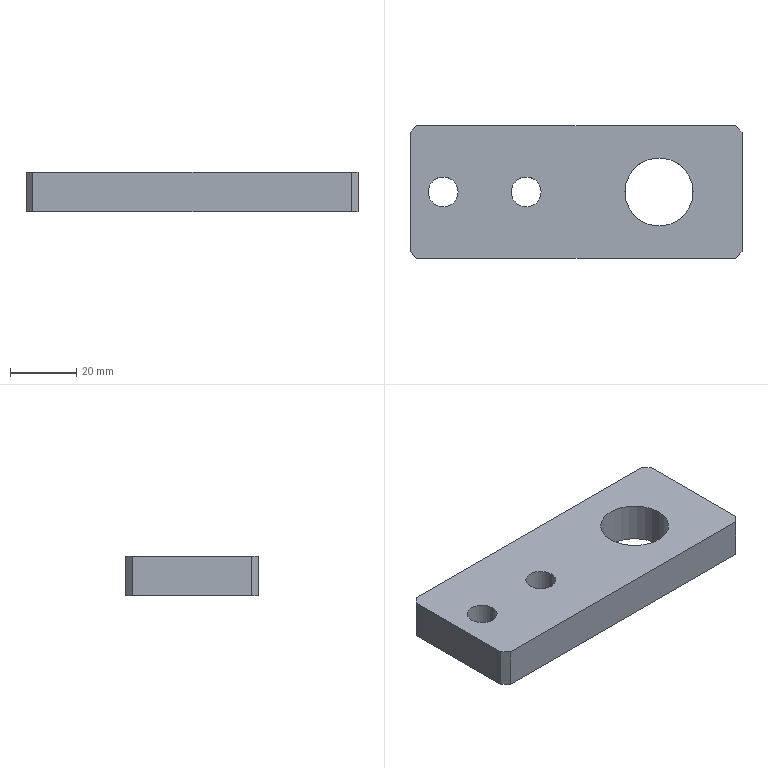Part | SolidWorks | features BaseBody 1 | 1 solid | 16 faces | box 100 x 40 x 12 mm | volume 42416 mm3 | plane 10 | cylinder 6 | commonest cylinder face diameters 9 x4 20.5 x2
STEP:
#1=CARTESIAN_POINT('',(-19.5,0.,0.));
#2=VERTEX_POINT('',#1);
#3=CARTESIAN_POINT('',(-10.5,0.,0.));
#4=VERTEX_POINT('',#3);
#5=CARTESIAN_POINT('',(-15.,0.,0.));
#6=DIRECTION('',(0.,0.,1.));
#7=DIRECTION('',(1.,0.,0.));
#8=AXIS2_PLACEMENT_3D('',#5,#6,#7);
#9=CIRCLE('',#8,4.5);
#10=EDGE_CURVE('',#2,#4,#9,.T.);
#11=ORIENTED_EDGE('',*,*,#10,.F.);
#12=CARTESIAN_POINT('',(-19.5,0.,12.));
#13=VERTEX_POINT('',#12);
#14=CARTESIAN_POINT('',(-19.5,0.,12.));
#15=DIRECTION('',(0.,0.,1.));
#16=VECTOR('',#15,1000.);
#17=LINE('',#14,#16);
#18=EDGE_CURVE('',#2,#13,#17,.T.);
#19=ORIENTED_EDGE('',*,*,#18,.T.);
#20=CARTESIAN_POINT('',(-10.5,0.,12.));
#21=VERTEX_POINT('',#20);
#22=CARTESIAN_POINT('',(-15.,0.,12.));
#23=DIRECTION('',(0.,0.,-1.));
#24=DIRECTION('',(1.,0.,0.));
#25=AXIS2_PLACEMENT_3D('',#22,#23,#24);
#26=CIRCLE('',#25,4.5);
#27=EDGE_CURVE('',#21,#13,#26,.T.);
#28=ORIENTED_EDGE('',*,*,#27,.F.);
#29=CARTESIAN_POINT('',(-10.5,0.,12.));
#30=DIRECTION('',(0.,0.,1.));
#31=VECTOR('',#30,1000.);
#32=LINE('',#29,#31);
#33=EDGE_CURVE('',#4,#21,#32,.T.);
#34=ORIENTED_EDGE('',*,*,#33,.F.);
#35=EDGE_LOOP('',(#11,#19,#28,#34));
#36=FACE_OUTER_BOUND('',#35,.T.);
#37=CARTESIAN_POINT('',(-15.,0.,12.));
#38=DIRECTION('',(0.,0.,1.));
#39=DIRECTION('',(1.,0.,0.));
#40=AXIS2_PLACEMENT_3D('',#37,#38,#39);
#41=CYLINDRICAL_SURFACE('',#40,4.5);
#42=ADVANCED_FACE('',(#36),#41,.F.);
#43=CARTESIAN_POINT('',(-44.5,0.,0.));
#44=VERTEX_POINT('',#43);
#45=CARTESIAN_POINT('',(-35.5,0.,0.));
#46=VERTEX_POINT('',#45);
#47=CARTESIAN_POINT('',(-40.,0.,0.));
#48=DIRECTION('',(0.,0.,1.));
#49=DIRECTION('',(1.,0.,0.));
#50=AXIS2_PLACEMENT_3D('',#47,#48,#49);
#51=CIRCLE('',#50,4.5);
#52=EDGE_CURVE('',#44,#46,#51,.T.);
#53=ORIENTED_EDGE('',*,*,#52,.F.);
#54=CARTESIAN_POINT('',(-44.5,0.,12.));
#55=VERTEX_POINT('',#54);
#56=CARTESIAN_POINT('',(-44.5,0.,12.));
#57=DIRECTION('',(0.,0.,1.));
#58=VECTOR('',#57,1000.);
#59=LINE('',#56,#58);
#60=EDGE_CURVE('',#44,#55,#59,.T.);
#61=ORIENTED_EDGE('',*,*,#60,.T.);
#62=CARTESIAN_POINT('',(-35.5,0.,12.));
#63=VERTEX_POINT('',#62);
#64=CARTESIAN_POINT('',(-40.,0.,12.));
#65=DIRECTION('',(0.,0.,-1.));
#66=DIRECTION('',(1.,0.,0.));
#67=AXIS2_PLACEMENT_3D('',#64,#65,#66);
#68=CIRCLE('',#67,4.5);
#69=EDGE_CURVE('',#63,#55,#68,.T.);
#70=ORIENTED_EDGE('',*,*,#69,.F.);
#71=CARTESIAN_POINT('',(-35.5,0.,12.));
#72=DIRECTION('',(0.,0.,1.));
#73=VECTOR('',#72,1000.);
#74=LINE('',#71,#73);
#75=EDGE_CURVE('',#46,#63,#74,.T.);
#76=ORIENTED_EDGE('',*,*,#75,.F.);
#77=EDGE_LOOP('',(#53,#61,#70,#76));
#78=FACE_OUTER_BOUND('',#77,.T.);
#79=CARTESIAN_POINT('',(-40.,0.,12.));
#80=DIRECTION('',(0.,0.,1.));
#81=DIRECTION('',(1.,0.,0.));
#82=AXIS2_PLACEMENT_3D('',#79,#80,#81);
#83=CYLINDRICAL_SURFACE('',#82,4.5);
#84=ADVANCED_FACE('',(#78),#83,.F.);
#85=CARTESIAN_POINT('',(14.75,0.,0.));
#86=VERTEX_POINT('',#85);
#87=CARTESIAN_POINT('',(35.25,0.,0.));
#88=VERTEX_POINT('',#87);
#89=CARTESIAN_POINT('',(25.,0.,0.));
#90=DIRECTION('',(0.,0.,1.));
#91=DIRECTION('',(1.,0.,0.));
#92=AXIS2_PLACEMENT_3D('',#89,#90,#91);
#93=CIRCLE('',#92,10.25);
#94=EDGE_CURVE('',#86,#88,#93,.T.);
#95=ORIENTED_EDGE('',*,*,#94,.F.);
#96=CARTESIAN_POINT('',(14.75,0.,12.));
#97=VERTEX_POINT('',#96);
#98=CARTESIAN_POINT('',(14.75,0.,12.));
#99=DIRECTION('',(0.,0.,1.));
#100=VECTOR('',#99,1000.);
#101=LINE('',#98,#100);
#102=EDGE_CURVE('',#86,#97,#101,.T.);
#103=ORIENTED_EDGE('',*,*,#102,.T.);
#104=CARTESIAN_POINT('',(35.25,0.,12.));
#105=VERTEX_POINT('',#104);
#106=CARTESIAN_POINT('',(25.,0.,12.));
#107=DIRECTION('',(0.,0.,-1.));
#108=DIRECTION('',(1.,0.,0.));
#109=AXIS2_PLACEMENT_3D('',#106,#107,#108);
#110=CIRCLE('',#109,10.25);
#111=EDGE_CURVE('',#105,#97,#110,.T.);
#112=ORIENTED_EDGE('',*,*,#111,.F.);
#113=CARTESIAN_POINT('',(35.25,0.,12.));
#114=DIRECTION('',(0.,0.,1.));
#115=VECTOR('',#114,1000.);
#116=LINE('',#113,#115);
#117=EDGE_CURVE('',#88,#105,#116,.T.);
#118=ORIENTED_EDGE('',*,*,#117,.F.);
#119=EDGE_LOOP('',(#95,#103,#112,#118));
#120=FACE_OUTER_BOUND('',#119,.T.);
#121=CARTESIAN_POINT('',(25.,0.,12.));
#122=DIRECTION('',(0.,0.,1.));
#123=DIRECTION('',(1.,0.,0.));
#124=AXIS2_PLACEMENT_3D('',#121,#122,#123);
#125=CYLINDRICAL_SURFACE('',#124,10.25);
#126=ADVANCED_FACE('',(#120),#125,.F.);
#127=CARTESIAN_POINT('',(-48.,-20.,12.));
#128=VERTEX_POINT('',#127);
#129=CARTESIAN_POINT('',(48.,-20.,12.));
#130=VERTEX_POINT('',#129);
#131=CARTESIAN_POINT('',(0.,-20.,12.));
#132=DIRECTION('',(1.,0.,0.));
#133=VECTOR('',#132,1000.);
#134=LINE('',#131,#133);
#135=EDGE_CURVE('',#128,#130,#134,.T.);
#136=ORIENTED_EDGE('',*,*,#135,.T.);
#137=CARTESIAN_POINT('',(50.,-18.,12.));
#138=VERTEX_POINT('',#137);
#139=CARTESIAN_POINT('',(48.,-20.,12.));
#140=DIRECTION('',(0.7071,0.7071,0.));
#141=VECTOR('',#140,1000.);
#142=LINE('',#139,#141);
#143=EDGE_CURVE('',#130,#138,#142,.T.);
#144=ORIENTED_EDGE('',*,*,#143,.T.);
#145=CARTESIAN_POINT('',(50.,18.,12.));
#146=VERTEX_POINT('',#145);
#147=CARTESIAN_POINT('',(50.,0.,12.));
#148=DIRECTION('',(0.,1.,0.));
#149=VECTOR('',#148,1000.);
#150=LINE('',#147,#149);
#151=EDGE_CURVE('',#138,#146,#150,.T.);
#152=ORIENTED_EDGE('',*,*,#151,.T.);
#153=CARTESIAN_POINT('',(48.,20.,12.));
#154=VERTEX_POINT('',#153);
#155=CARTESIAN_POINT('',(50.,18.,12.));
#156=DIRECTION('',(-0.7071,0.7071,0.));
#157=VECTOR('',#156,1000.);
#158=LINE('',#155,#157);
#159=EDGE_CURVE('',#146,#154,#158,.T.);
#160=ORIENTED_EDGE('',*,*,#159,.T.);
#161=CARTESIAN_POINT('',(-48.,20.,12.));
#162=VERTEX_POINT('',#161);
#163=CARTESIAN_POINT('',(0.,20.,12.));
#164=DIRECTION('',(-1.,0.,0.));
#165=VECTOR('',#164,1000.);
#166=LINE('',#163,#165);
#167=EDGE_CURVE('',#154,#162,#166,.T.);
#168=ORIENTED_EDGE('',*,*,#167,.T.);
#169=CARTESIAN_POINT('',(-50.,18.,12.));
#170=VERTEX_POINT('',#169);
#171=CARTESIAN_POINT('',(-48.,20.,12.));
#172=DIRECTION('',(-0.7071,-0.7071,0.));
#173=VECTOR('',#172,1000.);
#174=LINE('',#171,#173);
#175=EDGE_CURVE('',#162,#170,#174,.T.);
#176=ORIENTED_EDGE('',*,*,#175,.T.);
#177=CARTESIAN_POINT('',(-50.,-18.,12.));
#178=VERTEX_POINT('',#177);
#179=CARTESIAN_POINT('',(-50.,0.,12.));
#180=DIRECTION('',(0.,-1.,0.));
#181=VECTOR('',#180,1000.);
#182=LINE('',#179,#181);
#183=EDGE_CURVE('',#170,#178,#182,.T.);
#184=ORIENTED_EDGE('',*,*,#183,.T.);
#185=CARTESIAN_POINT('',(-50.,-18.,12.));
#186=DIRECTION('',(0.7071,-0.7071,0.));
#187=VECTOR('',#186,1000.);
#188=LINE('',#185,#187);
#189=EDGE_CURVE('',#178,#128,#188,.T.);
#190=ORIENTED_EDGE('',*,*,#189,.T.);
#191=EDGE_LOOP('',(#136,#144,#152,#160,#168,#176,#184,#190));
#192=FACE_OUTER_BOUND('',#191,.T.);
#193=ORIENTED_EDGE('',*,*,#27,.T.);
#194=CARTESIAN_POINT('',(-15.,0.,12.));
#195=DIRECTION('',(0.,0.,-1.));
#196=DIRECTION('',(1.,0.,0.));
#197=AXIS2_PLACEMENT_3D('',#194,#195,#196);
#198=CIRCLE('',#197,4.5);
#199=EDGE_CURVE('',#13,#21,#198,.T.);
#200=ORIENTED_EDGE('',*,*,#199,.T.);
#201=EDGE_LOOP('',(#193,#200));
#202=FACE_BOUND('',#201,.T.);
#203=ORIENTED_EDGE('',*,*,#69,.T.);
#204=CARTESIAN_POINT('',(-40.,0.,12.));
#205=DIRECTION('',(0.,0.,-1.));
#206=DIRECTION('',(1.,0.,0.));
#207=AXIS2_PLACEMENT_3D('',#204,#205,#206);
#208=CIRCLE('',#207,4.5);
#209=EDGE_CURVE('',#55,#63,#208,.T.);
#210=ORIENTED_EDGE('',*,*,#209,.T.);
#211=EDGE_LOOP('',(#203,#210));
#212=FACE_BOUND('',#211,.T.);
#213=ORIENTED_EDGE('',*,*,#111,.T.);
#214=CARTESIAN_POINT('',(25.,0.,12.));
#215=DIRECTION('',(0.,0.,-1.));
#216=DIRECTION('',(1.,0.,0.));
#217=AXIS2_PLACEMENT_3D('',#214,#215,#216);
#218=CIRCLE('',#217,10.25);
#219=EDGE_CURVE('',#97,#105,#218,.T.);
#220=ORIENTED_EDGE('',*,*,#219,.T.);
#221=EDGE_LOOP('',(#213,#220));
#222=FACE_BOUND('',#221,.T.);
#223=CARTESIAN_POINT('',(0.,0.,12.));
#224=DIRECTION('',(0.,0.,1.));
#225=DIRECTION('',(1.,0.,0.));
#226=AXIS2_PLACEMENT_3D('',#223,#224,#225);
#227=PLANE('',#226);
#228=ADVANCED_FACE('',(#192,#202,#212,#222),#227,.T.);
#229=CARTESIAN_POINT('',(48.,-20.,0.));
#230=VERTEX_POINT('',#229);
#231=CARTESIAN_POINT('',(48.,-20.,12.));
#232=DIRECTION('',(0.,0.,1.));
#233=VECTOR('',#232,1000.);
#234=LINE('',#231,#233);
#235=EDGE_CURVE('',#230,#130,#234,.T.);
#236=ORIENTED_EDGE('',*,*,#235,.F.);
#237=CARTESIAN_POINT('',(50.,-18.,0.));
#238=VERTEX_POINT('',#237);
#239=CARTESIAN_POINT('',(50.,-18.,0.));
#240=DIRECTION('',(-0.7071,-0.7071,0.));
#241=VECTOR('',#240,1000.);
#242=LINE('',#239,#241);
#243=EDGE_CURVE('',#238,#230,#242,.T.);
#244=ORIENTED_EDGE('',*,*,#243,.F.);
#245=CARTESIAN_POINT('',(50.,-18.,12.));
#246=DIRECTION('',(0.,0.,-1.));
#247=VECTOR('',#246,1000.);
#248=LINE('',#245,#247);
#249=EDGE_CURVE('',#138,#238,#248,.T.);
#250=ORIENTED_EDGE('',*,*,#249,.F.);
#251=ORIENTED_EDGE('',*,*,#143,.F.);
#252=EDGE_LOOP('',(#236,#244,#250,#251));
#253=FACE_OUTER_BOUND('',#252,.T.);
#254=CARTESIAN_POINT('',(50.,-18.,12.));
#255=DIRECTION('',(-0.7071,0.7071,0.));
#256=DIRECTION('',(-0.7071,-0.7071,0.));
#257=AXIS2_PLACEMENT_3D('',#254,#255,#256);
#258=PLANE('',#257);
#259=ADVANCED_FACE('',(#253),#258,.F.);
#260=ORIENTED_EDGE('',*,*,#235,.T.);
#261=ORIENTED_EDGE('',*,*,#135,.F.);
#262=CARTESIAN_POINT('',(-48.,-20.,0.));
#263=VERTEX_POINT('',#262);
#264=CARTESIAN_POINT('',(-48.,-20.,12.));
#265=DIRECTION('',(0.,0.,1.));
#266=VECTOR('',#265,1000.);
#267=LINE('',#264,#266);
#268=EDGE_CURVE('',#263,#128,#267,.T.);
#269=ORIENTED_EDGE('',*,*,#268,.F.);
#270=CARTESIAN_POINT('',(-50.,-20.,0.));
#271=DIRECTION('',(-1.,0.,0.));
#272=VECTOR('',#271,1000.);
#273=LINE('',#270,#272);
#274=EDGE_CURVE('',#230,#263,#273,.T.);
#275=ORIENTED_EDGE('',*,*,#274,.F.);
#276=EDGE_LOOP('',(#260,#261,#269,#275));
#277=FACE_OUTER_BOUND('',#276,.T.);
#278=CARTESIAN_POINT('',(-50.,-20.,12.));
#279=DIRECTION('',(0.,1.,0.));
#280=DIRECTION('',(0.,0.,1.));
#281=AXIS2_PLACEMENT_3D('',#278,#279,#280);
#282=PLANE('',#281);
#283=ADVANCED_FACE('',(#277),#282,.F.);
#284=CARTESIAN_POINT('',(-50.,-18.,0.));
#285=VERTEX_POINT('',#284);
#286=CARTESIAN_POINT('',(-50.,-18.,12.));
#287=DIRECTION('',(0.,0.,1.));
#288=VECTOR('',#287,1000.);
#289=LINE('',#286,#288);
#290=EDGE_CURVE('',#285,#178,#289,.T.);
#291=ORIENTED_EDGE('',*,*,#290,.F.);
#292=CARTESIAN_POINT('',(-48.,-20.,0.));
#293=DIRECTION('',(-0.7071,0.7071,0.));
#294=VECTOR('',#293,1000.);
#295=LINE('',#292,#294);
#296=EDGE_CURVE('',#263,#285,#295,.T.);
#297=ORIENTED_EDGE('',*,*,#296,.F.);
#298=ORIENTED_EDGE('',*,*,#268,.T.);
#299=ORIENTED_EDGE('',*,*,#189,.F.);
#300=EDGE_LOOP('',(#291,#297,#298,#299));
#301=FACE_OUTER_BOUND('',#300,.T.);
#302=CARTESIAN_POINT('',(-48.,-20.,12.));
#303=DIRECTION('',(0.7071,0.7071,0.));
#304=DIRECTION('',(-0.7071,0.7071,0.));
#305=AXIS2_PLACEMENT_3D('',#302,#303,#304);
#306=PLANE('',#305);
#307=ADVANCED_FACE('',(#301),#306,.F.);
#308=CARTESIAN_POINT('',(-50.,18.,0.));
#309=VERTEX_POINT('',#308);
#310=CARTESIAN_POINT('',(-50.,18.,12.));
#311=DIRECTION('',(0.,0.,1.));
#312=VECTOR('',#311,1000.);
#313=LINE('',#310,#312);
#314=EDGE_CURVE('',#309,#170,#313,.T.);
#315=ORIENTED_EDGE('',*,*,#314,.F.);
#316=CARTESIAN_POINT('',(-50.,20.,0.));
#317=DIRECTION('',(0.,1.,0.));
#318=VECTOR('',#317,1000.);
#319=LINE('',#316,#318);
#320=EDGE_CURVE('',#285,#309,#319,.T.);
#321=ORIENTED_EDGE('',*,*,#320,.F.);
#322=ORIENTED_EDGE('',*,*,#290,.T.);
#323=ORIENTED_EDGE('',*,*,#183,.F.);
#324=EDGE_LOOP('',(#315,#321,#322,#323));
#325=FACE_OUTER_BOUND('',#324,.T.);
#326=CARTESIAN_POINT('',(-50.,20.,12.));
#327=DIRECTION('',(1.,0.,0.));
#328=DIRECTION('',(0.,0.,-1.));
#329=AXIS2_PLACEMENT_3D('',#326,#327,#328);
#330=PLANE('',#329);
#331=ADVANCED_FACE('',(#325),#330,.F.);
#332=CARTESIAN_POINT('',(-48.,20.,0.));
#333=VERTEX_POINT('',#332);
#334=CARTESIAN_POINT('',(-48.,20.,12.));
#335=DIRECTION('',(0.,0.,1.));
#336=VECTOR('',#335,1000.);
#337=LINE('',#334,#336);
#338=EDGE_CURVE('',#333,#162,#337,.T.);
#339=ORIENTED_EDGE('',*,*,#338,.F.);
#340=CARTESIAN_POINT('',(-50.,18.,0.));
#341=DIRECTION('',(0.7071,0.7071,0.));
#342=VECTOR('',#341,1000.);
#343=LINE('',#340,#342);
#344=EDGE_CURVE('',#309,#333,#343,.T.);
#345=ORIENTED_EDGE('',*,*,#344,.F.);
#346=ORIENTED_EDGE('',*,*,#314,.T.);
#347=ORIENTED_EDGE('',*,*,#175,.F.);
#348=EDGE_LOOP('',(#339,#345,#346,#347));
#349=FACE_OUTER_BOUND('',#348,.T.);
#350=CARTESIAN_POINT('',(-50.,18.,12.));
#351=DIRECTION('',(0.7071,-0.7071,0.));
#352=DIRECTION('',(0.7071,0.7071,0.));
#353=AXIS2_PLACEMENT_3D('',#350,#351,#352);
#354=PLANE('',#353);
#355=ADVANCED_FACE('',(#349),#354,.F.);
#356=CARTESIAN_POINT('',(48.,20.,0.));
#357=VERTEX_POINT('',#356);
#358=CARTESIAN_POINT('',(48.,20.,12.));
#359=DIRECTION('',(0.,0.,1.));
#360=VECTOR('',#359,1000.);
#361=LINE('',#358,#360);
#362=EDGE_CURVE('',#357,#154,#361,.T.);
#363=ORIENTED_EDGE('',*,*,#362,.F.);
#364=CARTESIAN_POINT('',(-50.,20.,0.));
#365=DIRECTION('',(1.,0.,0.));
#366=VECTOR('',#365,1000.);
#367=LINE('',#364,#366);
#368=EDGE_CURVE('',#333,#357,#367,.T.);
#369=ORIENTED_EDGE('',*,*,#368,.F.);
#370=ORIENTED_EDGE('',*,*,#338,.T.);
#371=ORIENTED_EDGE('',*,*,#167,.F.);
#372=EDGE_LOOP('',(#363,#369,#370,#371));
#373=FACE_OUTER_BOUND('',#372,.T.);
#374=CARTESIAN_POINT('',(-50.,20.,12.));
#375=DIRECTION('',(0.,-1.,0.));
#376=DIRECTION('',(0.,0.,-1.));
#377=AXIS2_PLACEMENT_3D('',#374,#375,#376);
#378=PLANE('',#377);
#379=ADVANCED_FACE('',(#373),#378,.F.);
#380=CARTESIAN_POINT('',(50.,18.,0.));
#381=VERTEX_POINT('',#380);
#382=CARTESIAN_POINT('',(50.,18.,12.));
#383=DIRECTION('',(0.,0.,1.));
#384=VECTOR('',#383,1000.);
#385=LINE('',#382,#384);
#386=EDGE_CURVE('',#381,#146,#385,.T.);
#387=ORIENTED_EDGE('',*,*,#386,.F.);
#388=CARTESIAN_POINT('',(48.,20.,0.));
#389=DIRECTION('',(0.7071,-0.7071,0.));
#390=VECTOR('',#389,1000.);
#391=LINE('',#388,#390);
#392=EDGE_CURVE('',#357,#381,#391,.T.);
#393=ORIENTED_EDGE('',*,*,#392,.F.);
#394=ORIENTED_EDGE('',*,*,#362,.T.);
#395=ORIENTED_EDGE('',*,*,#159,.F.);
#396=EDGE_LOOP('',(#387,#393,#394,#395));
#397=FACE_OUTER_BOUND('',#396,.T.);
#398=CARTESIAN_POINT('',(48.,20.,12.));
#399=DIRECTION('',(-0.7071,-0.7071,0.));
#400=DIRECTION('',(0.7071,-0.7071,0.));
#401=AXIS2_PLACEMENT_3D('',#398,#399,#400);
#402=PLANE('',#401);
#403=ADVANCED_FACE('',(#397),#402,.F.);
#404=ORIENTED_EDGE('',*,*,#386,.T.);
#405=ORIENTED_EDGE('',*,*,#151,.F.);
#406=ORIENTED_EDGE('',*,*,#249,.T.);
#407=CARTESIAN_POINT('',(50.,20.,0.));
#408=DIRECTION('',(0.,-1.,0.));
#409=VECTOR('',#408,1000.);
#410=LINE('',#407,#409);
#411=EDGE_CURVE('',#381,#238,#410,.T.);
#412=ORIENTED_EDGE('',*,*,#411,.F.);
#413=EDGE_LOOP('',(#404,#405,#406,#412));
#414=FACE_OUTER_BOUND('',#413,.T.);
#415=CARTESIAN_POINT('',(50.,20.,12.));
#416=DIRECTION('',(-1.,0.,0.));
#417=DIRECTION('',(0.,0.,1.));
#418=AXIS2_PLACEMENT_3D('',#415,#416,#417);
#419=PLANE('',#418);
#420=ADVANCED_FACE('',(#414),#419,.F.);
#421=ORIENTED_EDGE('',*,*,#18,.F.);
#422=CARTESIAN_POINT('',(-15.,0.,0.));
#423=DIRECTION('',(0.,0.,1.));
#424=DIRECTION('',(1.,0.,0.));
#425=AXIS2_PLACEMENT_3D('',#422,#423,#424);
#426=CIRCLE('',#425,4.5);
#427=EDGE_CURVE('',#4,#2,#426,.T.);
#428=ORIENTED_EDGE('',*,*,#427,.F.);
#429=ORIENTED_EDGE('',*,*,#33,.T.);
#430=ORIENTED_EDGE('',*,*,#199,.F.);
#431=EDGE_LOOP('',(#421,#428,#429,#430));
#432=FACE_OUTER_BOUND('',#431,.T.);
#433=CARTESIAN_POINT('',(-15.,0.,12.));
#434=DIRECTION('',(0.,0.,1.));
#435=DIRECTION('',(1.,0.,0.));
#436=AXIS2_PLACEMENT_3D('',#433,#434,#435);
#437=CYLINDRICAL_SURFACE('',#436,4.5);
#438=ADVANCED_FACE('',(#432),#437,.F.);
#439=ORIENTED_EDGE('',*,*,#60,.F.);
#440=CARTESIAN_POINT('',(-40.,0.,0.));
#441=DIRECTION('',(0.,0.,1.));
#442=DIRECTION('',(1.,0.,0.));
#443=AXIS2_PLACEMENT_3D('',#440,#441,#442);
#444=CIRCLE('',#443,4.5);
#445=EDGE_CURVE('',#46,#44,#444,.T.);
#446=ORIENTED_EDGE('',*,*,#445,.F.);
#447=ORIENTED_EDGE('',*,*,#75,.T.);
#448=ORIENTED_EDGE('',*,*,#209,.F.);
#449=EDGE_LOOP('',(#439,#446,#447,#448));
#450=FACE_OUTER_BOUND('',#449,.T.);
#451=CARTESIAN_POINT('',(-40.,0.,12.));
#452=DIRECTION('',(0.,0.,1.));
#453=DIRECTION('',(1.,0.,0.));
#454=AXIS2_PLACEMENT_3D('',#451,#452,#453);
#455=CYLINDRICAL_SURFACE('',#454,4.5);
#456=ADVANCED_FACE('',(#450),#455,.F.);
#457=ORIENTED_EDGE('',*,*,#102,.F.);
#458=CARTESIAN_POINT('',(25.,0.,0.));
#459=DIRECTION('',(0.,0.,1.));
#460=DIRECTION('',(1.,0.,0.));
#461=AXIS2_PLACEMENT_3D('',#458,#459,#460);
#462=CIRCLE('',#461,10.25);
#463=EDGE_CURVE('',#88,#86,#462,.T.);
#464=ORIENTED_EDGE('',*,*,#463,.F.);
#465=ORIENTED_EDGE('',*,*,#117,.T.);
#466=ORIENTED_EDGE('',*,*,#219,.F.);
#467=EDGE_LOOP('',(#457,#464,#465,#466));
#468=FACE_OUTER_BOUND('',#467,.T.);
#469=CARTESIAN_POINT('',(25.,0.,12.));
#470=DIRECTION('',(0.,0.,1.));
#471=DIRECTION('',(1.,0.,0.));
#472=AXIS2_PLACEMENT_3D('',#469,#470,#471);
#473=CYLINDRICAL_SURFACE('',#472,10.25);
#474=ADVANCED_FACE('',(#468),#473,.F.);
#475=ORIENTED_EDGE('',*,*,#392,.T.);
#476=ORIENTED_EDGE('',*,*,#411,.T.);
#477=ORIENTED_EDGE('',*,*,#243,.T.);
#478=ORIENTED_EDGE('',*,*,#274,.T.);
#479=ORIENTED_EDGE('',*,*,#296,.T.);
#480=ORIENTED_EDGE('',*,*,#320,.T.);
#481=ORIENTED_EDGE('',*,*,#344,.T.);
#482=ORIENTED_EDGE('',*,*,#368,.T.);
#483=EDGE_LOOP('',(#475,#476,#477,#478,#479,#480,#481,#482));
#484=FACE_OUTER_BOUND('',#483,.T.);
#485=ORIENTED_EDGE('',*,*,#427,.T.);
#486=ORIENTED_EDGE('',*,*,#10,.T.);
#487=EDGE_LOOP('',(#485,#486));
#488=FACE_BOUND('',#487,.T.);
#489=ORIENTED_EDGE('',*,*,#445,.T.);
#490=ORIENTED_EDGE('',*,*,#52,.T.);
#491=EDGE_LOOP('',(#489,#490));
#492=FACE_BOUND('',#491,.T.);
#493=ORIENTED_EDGE('',*,*,#463,.T.);
#494=ORIENTED_EDGE('',*,*,#94,.T.);
#495=EDGE_LOOP('',(#493,#494));
#496=FACE_BOUND('',#495,.T.);
#497=CARTESIAN_POINT('',(0.,0.,0.));
#498=DIRECTION('',(0.,0.,1.));
#499=DIRECTION('',(1.,0.,0.));
#500=AXIS2_PLACEMENT_3D('',#497,#498,#499);
#501=PLANE('',#500);
#502=ADVANCED_FACE('',(#484,#488,#492,#496),#501,.F.);
#503=CLOSED_SHELL('',(#42,#84,#126,#228,#259,#283,#307,#331,#355,#379,#403,#420,#438,#456,#474,#502));
#504=MANIFOLD_SOLID_BREP('',#503);
#505=CARTESIAN_POINT('',(0.,0.,0.));
#506=DIRECTION('',(0.,0.,1.));
#507=DIRECTION('',(1.,0.,0.));
#508=AXIS2_PLACEMENT_3D('',#505,#506,#507);
#509=(LENGTH_UNIT()NAMED_UNIT(*)SI_UNIT(.MILLI.,.METRE.));
#510=UNCERTAINTY_MEASURE_WITH_UNIT(LENGTH_MEASURE(0.00001),#509,'','');
#511=(NAMED_UNIT(*)PLANE_ANGLE_UNIT()SI_UNIT($,.RADIAN.));
#512=(NAMED_UNIT(*)SI_UNIT($,.STERADIAN.)SOLID_ANGLE_UNIT());
#513=(GEOMETRIC_REPRESENTATION_CONTEXT(3)GLOBAL_UNCERTAINTY_ASSIGNED_CONTEXT((#510))GLOBAL_UNIT_ASSIGNED_CONTEXT((#509,#511,#512))REPRESENTATION_CONTEXT('',''));
#514=ADVANCED_BREP_SHAPE_REPRESENTATION('',(#504,#508),#513);